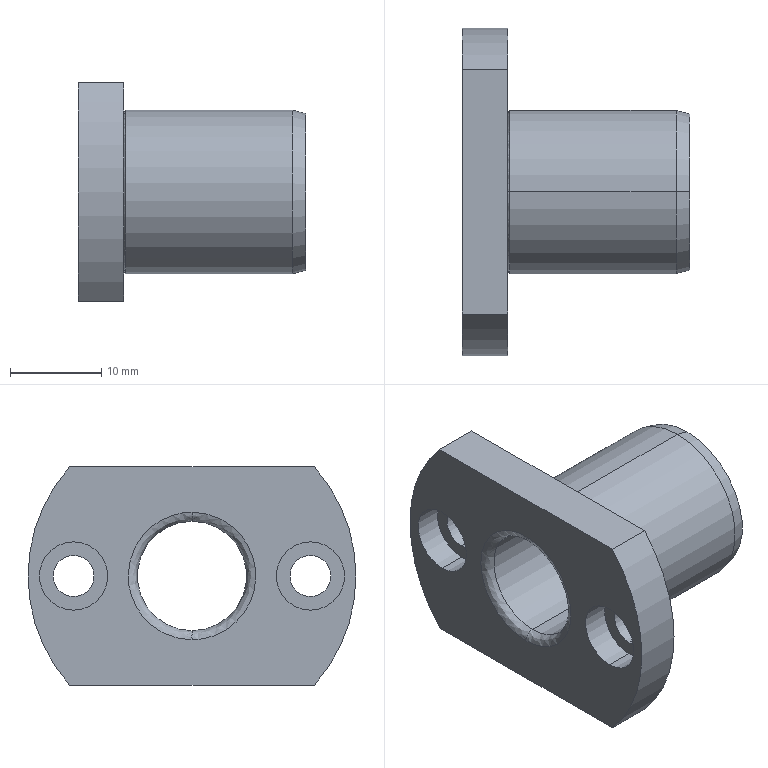Part | STEP file | SHTNZ12-25_1 | 1 solid | 29 faces | box 25 x 36 x 24 mm | volume 5866 mm3 | cylinder 14 | plane 7 | spline 4 | cone 4 | commonest cylinder face diameters 4.5 x4 7.5 x4 12 x2 18 x2 36 x2